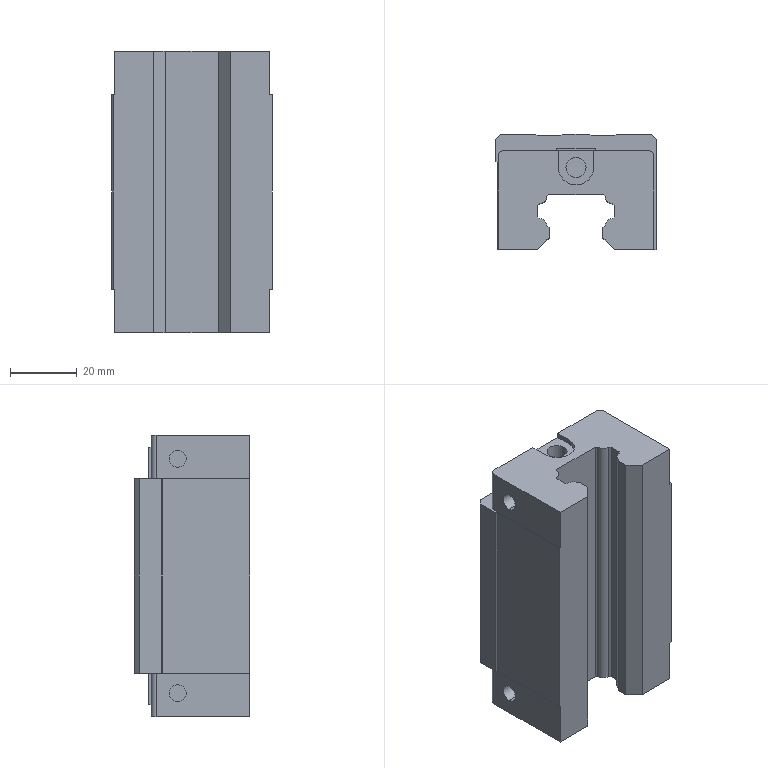Part | SolidWorks | features ICE 12, HoleWzd 5, RevCut 4, Chamfer 3, Draft 3, Extrusion 1, Fillet 1 | 1 solid | 121 faces | box 48 x 34.5 x 84 mm | volume 100896 mm3 | plane 72 | cylinder 41 | cone 8 | commonest cylinder face diameters 6 x12 5 x8 1 x7 3 x4 4.6 x4 7.3 x4